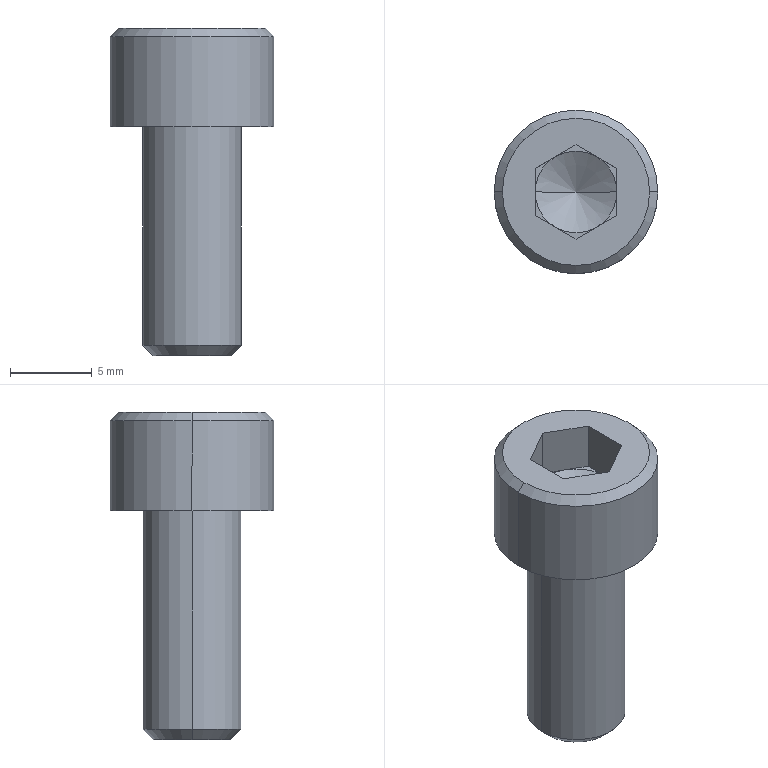Part | NX | features BREP 1 | 1 solid | 25 faces | box 10 x 10 x 20 mm | volume 785.579 mm3 | plane 15 | cone 6 | cylinder 4 | commonest cylinder face diameters 6 x2 10 x2
STEP:
#1=CARTESIAN_POINT('',(0.,0.,1.557));
#2=VERTEX_POINT('',#1);
#3=CARTESIAN_POINT('',(2.5,0.,3.));
#4=VERTEX_POINT('',#3);
#5=CARTESIAN_POINT('',(0.,0.,1.557));
#6=DIRECTION('',(0.866,0.,0.5));
#7=VECTOR('',#6,1000.);
#8=LINE('',#5,#7);
#9=EDGE_CURVE('',#2,#4,#8,.T.);
#10=ORIENTED_EDGE('',*,*,#9,.F.);
#11=CARTESIAN_POINT('',(-2.5,0.,3.));
#12=VERTEX_POINT('',#11);
#13=CARTESIAN_POINT('',(0.,0.,1.557));
#14=DIRECTION('',(-0.866,0.,0.5));
#15=VECTOR('',#14,1000.);
#16=LINE('',#13,#15);
#17=EDGE_CURVE('',#2,#12,#16,.T.);
#18=ORIENTED_EDGE('',*,*,#17,.T.);
#19=CARTESIAN_POINT('',(-1.25,-2.165,3.));
#20=VERTEX_POINT('',#19);
#21=CARTESIAN_POINT('',(0.,0.,3.));
#22=DIRECTION('',(0.,0.,1.));
#23=DIRECTION('',(1.,0.,0.));
#24=AXIS2_PLACEMENT_3D('',#21,#22,#23);
#25=CIRCLE('',#24,2.5);
#26=EDGE_CURVE('',#12,#20,#25,.T.);
#27=ORIENTED_EDGE('',*,*,#26,.T.);
#28=CARTESIAN_POINT('',(1.25,-2.165,3.));
#29=VERTEX_POINT('',#28);
#30=CARTESIAN_POINT('',(0.,0.,3.));
#31=DIRECTION('',(0.,0.,1.));
#32=DIRECTION('',(1.,0.,0.));
#33=AXIS2_PLACEMENT_3D('',#30,#31,#32);
#34=CIRCLE('',#33,2.5);
#35=EDGE_CURVE('',#20,#29,#34,.T.);
#36=ORIENTED_EDGE('',*,*,#35,.T.);
#37=CARTESIAN_POINT('',(0.,0.,3.));
#38=DIRECTION('',(0.,0.,1.));
#39=DIRECTION('',(1.,0.,0.));
#40=AXIS2_PLACEMENT_3D('',#37,#38,#39);
#41=CIRCLE('',#40,2.5);
#42=EDGE_CURVE('',#29,#4,#41,.T.);
#43=ORIENTED_EDGE('',*,*,#42,.T.);
#44=EDGE_LOOP('',(#10,#18,#27,#36,#43));
#45=FACE_BOUND('',#44,.T.);
#46=CARTESIAN_POINT('',(0.,0.,1001.557));
#47=DIRECTION('',(0.,0.,1.));
#48=DIRECTION('',(-1.,0.,0.));
#49=AXIS2_PLACEMENT_3D('',#46,#47,#48);
#50=CONICAL_SURFACE('',#49,1732.051,1.047);
#51=ADVANCED_FACE('',(#45),#50,.F.);
#52=CARTESIAN_POINT('',(5.,0.,0.));
#53=VERTEX_POINT('',#52);
#54=CARTESIAN_POINT('',(-5.,0.,0.));
#55=VERTEX_POINT('',#54);
#56=CARTESIAN_POINT('',(0.,0.,0.));
#57=DIRECTION('',(0.,0.,1.));
#58=DIRECTION('',(1.,0.,0.));
#59=AXIS2_PLACEMENT_3D('',#56,#57,#58);
#60=CIRCLE('',#59,5.);
#61=EDGE_CURVE('',#53,#55,#60,.T.);
#62=ORIENTED_EDGE('',*,*,#61,.T.);
#63=CARTESIAN_POINT('',(-5.,0.,5.5));
#64=VERTEX_POINT('',#63);
#65=CARTESIAN_POINT('',(-5.,0.,0.));
#66=DIRECTION('',(0.,0.,1.));
#67=VECTOR('',#66,1000.);
#68=LINE('',#65,#67);
#69=EDGE_CURVE('',#55,#64,#68,.T.);
#70=ORIENTED_EDGE('',*,*,#69,.T.);
#71=CARTESIAN_POINT('',(5.,0.,5.5));
#72=VERTEX_POINT('',#71);
#73=CARTESIAN_POINT('',(0.,0.,5.5));
#74=DIRECTION('',(0.,0.,1.));
#75=DIRECTION('',(1.,0.,0.));
#76=AXIS2_PLACEMENT_3D('',#73,#74,#75);
#77=CIRCLE('',#76,5.);
#78=EDGE_CURVE('',#72,#64,#77,.T.);
#79=ORIENTED_EDGE('',*,*,#78,.F.);
#80=CARTESIAN_POINT('',(5.,0.,0.));
#81=DIRECTION('',(0.,0.,1.));
#82=VECTOR('',#81,1000.);
#83=LINE('',#80,#82);
#84=EDGE_CURVE('',#53,#72,#83,.T.);
#85=ORIENTED_EDGE('',*,*,#84,.F.);
#86=EDGE_LOOP('',(#62,#70,#79,#85));
#87=FACE_BOUND('',#86,.T.);
#88=CARTESIAN_POINT('',(0.,0.,0.));
#89=DIRECTION('',(0.,0.,1.));
#90=DIRECTION('',(-1.,0.,0.));
#91=AXIS2_PLACEMENT_3D('',#88,#89,#90);
#92=CYLINDRICAL_SURFACE('',#91,5.);
#93=ADVANCED_FACE('',(#87),#92,.T.);
#94=CARTESIAN_POINT('',(4.5,0.,6.));
#95=VERTEX_POINT('',#94);
#96=CARTESIAN_POINT('',(-4.5,0.,6.));
#97=VERTEX_POINT('',#96);
#98=CARTESIAN_POINT('',(0.,0.,6.));
#99=DIRECTION('',(0.,0.,1.));
#100=DIRECTION('',(1.,0.,0.));
#101=AXIS2_PLACEMENT_3D('',#98,#99,#100);
#102=CIRCLE('',#101,4.5);
#103=EDGE_CURVE('',#95,#97,#102,.T.);
#104=ORIENTED_EDGE('',*,*,#103,.F.);
#105=CARTESIAN_POINT('',(5.,0.,5.5));
#106=DIRECTION('',(0.7071,0.,-0.7071));
#107=VECTOR('',#106,1000.);
#108=LINE('',#105,#107);
#109=EDGE_CURVE('',#72,#95,#108,.F.);
#110=ORIENTED_EDGE('',*,*,#109,.F.);
#111=ORIENTED_EDGE('',*,*,#78,.T.);
#112=CARTESIAN_POINT('',(-5.,0.,5.5));
#113=DIRECTION('',(-0.7071,0.,-0.7071));
#114=VECTOR('',#113,1000.);
#115=LINE('',#112,#114);
#116=EDGE_CURVE('',#64,#97,#115,.F.);
#117=ORIENTED_EDGE('',*,*,#116,.T.);
#118=EDGE_LOOP('',(#104,#110,#111,#117));
#119=FACE_BOUND('',#118,.T.);
#120=CARTESIAN_POINT('',(0.,0.,5.5));
#121=DIRECTION('',(0.,0.,-1.));
#122=DIRECTION('',(1.,0.,0.));
#123=AXIS2_PLACEMENT_3D('',#120,#121,#122);
#124=CONICAL_SURFACE('',#123,5.,0.7854);
#125=ADVANCED_FACE('',(#119),#124,.T.);
#126=CARTESIAN_POINT('',(2.386,0.,-14.));
#127=VERTEX_POINT('',#126);
#128=CARTESIAN_POINT('',(-2.386,0.,-14.));
#129=VERTEX_POINT('',#128);
#130=CARTESIAN_POINT('',(0.,0.,-14.));
#131=DIRECTION('',(0.,0.,1.));
#132=DIRECTION('',(1.,0.,0.));
#133=AXIS2_PLACEMENT_3D('',#130,#131,#132);
#134=CIRCLE('',#133,2.386);
#135=EDGE_CURVE('',#127,#129,#134,.T.);
#136=ORIENTED_EDGE('',*,*,#135,.T.);
#137=CARTESIAN_POINT('',(-3.,0.,-13.386));
#138=VERTEX_POINT('',#137);
#139=CARTESIAN_POINT('',(-2.386,0.,-14.));
#140=DIRECTION('',(-0.7071,0.,0.7071));
#141=VECTOR('',#140,1000.);
#142=LINE('',#139,#141);
#143=EDGE_CURVE('',#129,#138,#142,.T.);
#144=ORIENTED_EDGE('',*,*,#143,.T.);
#145=CARTESIAN_POINT('',(3.,0.,-13.386));
#146=VERTEX_POINT('',#145);
#147=CARTESIAN_POINT('',(0.,0.,-13.386));
#148=DIRECTION('',(0.,0.,1.));
#149=DIRECTION('',(1.,0.,0.));
#150=AXIS2_PLACEMENT_3D('',#147,#148,#149);
#151=CIRCLE('',#150,3.);
#152=EDGE_CURVE('',#146,#138,#151,.T.);
#153=ORIENTED_EDGE('',*,*,#152,.F.);
#154=CARTESIAN_POINT('',(2.386,0.,-14.));
#155=DIRECTION('',(0.7071,0.,0.7071));
#156=VECTOR('',#155,1000.);
#157=LINE('',#154,#156);
#158=EDGE_CURVE('',#127,#146,#157,.T.);
#159=ORIENTED_EDGE('',*,*,#158,.F.);
#160=EDGE_LOOP('',(#136,#144,#153,#159));
#161=FACE_BOUND('',#160,.T.);
#162=CARTESIAN_POINT('',(0.,0.,-14.));
#163=DIRECTION('',(0.,0.,1.));
#164=DIRECTION('',(-1.,0.,0.));
#165=AXIS2_PLACEMENT_3D('',#162,#163,#164);
#166=CONICAL_SURFACE('',#165,2.386,0.7854);
#167=ADVANCED_FACE('',(#161),#166,.T.);
#168=ORIENTED_EDGE('',*,*,#152,.T.);
#169=CARTESIAN_POINT('',(-3.,0.,0.));
#170=VERTEX_POINT('',#169);
#171=CARTESIAN_POINT('',(-3.,0.,-14.));
#172=DIRECTION('',(0.,0.,1.));
#173=VECTOR('',#172,1000.);
#174=LINE('',#171,#173);
#175=EDGE_CURVE('',#138,#170,#174,.T.);
#176=ORIENTED_EDGE('',*,*,#175,.T.);
#177=CARTESIAN_POINT('',(3.,0.,0.));
#178=VERTEX_POINT('',#177);
#179=CARTESIAN_POINT('',(0.,0.,0.));
#180=DIRECTION('',(0.,0.,1.));
#181=DIRECTION('',(1.,0.,0.));
#182=AXIS2_PLACEMENT_3D('',#179,#180,#181);
#183=CIRCLE('',#182,3.);
#184=EDGE_CURVE('',#178,#170,#183,.T.);
#185=ORIENTED_EDGE('',*,*,#184,.F.);
#186=CARTESIAN_POINT('',(3.,0.,-14.));
#187=DIRECTION('',(0.,0.,1.));
#188=VECTOR('',#187,1000.);
#189=LINE('',#186,#188);
#190=EDGE_CURVE('',#146,#178,#189,.T.);
#191=ORIENTED_EDGE('',*,*,#190,.F.);
#192=EDGE_LOOP('',(#168,#176,#185,#191));
#193=FACE_BOUND('',#192,.T.);
#194=CARTESIAN_POINT('',(0.,0.,-14.));
#195=DIRECTION('',(0.,0.,1.));
#196=DIRECTION('',(-1.,0.,0.));
#197=AXIS2_PLACEMENT_3D('',#194,#195,#196);
#198=CYLINDRICAL_SURFACE('',#197,3.);
#199=ADVANCED_FACE('',(#193),#198,.T.);
#200=CARTESIAN_POINT('',(1.25,2.165,3.));
#201=VERTEX_POINT('',#200);
#202=CARTESIAN_POINT('',(0.,0.,3.));
#203=DIRECTION('',(0.,0.,1.));
#204=DIRECTION('',(1.,0.,0.));
#205=AXIS2_PLACEMENT_3D('',#202,#203,#204);
#206=CIRCLE('',#205,2.5);
#207=EDGE_CURVE('',#4,#201,#206,.T.);
#208=ORIENTED_EDGE('',*,*,#207,.F.);
#209=CARTESIAN_POINT('',(2.5,1.443,3.));
#210=VERTEX_POINT('',#209);
#211=CARTESIAN_POINT('',(2.5,-1.443,3.));
#212=DIRECTION('',(0.,1.,0.));
#213=VECTOR('',#212,1000.);
#214=LINE('',#211,#213);
#215=EDGE_CURVE('',#4,#210,#214,.T.);
#216=ORIENTED_EDGE('',*,*,#215,.T.);
#217=CARTESIAN_POINT('',(2.5,1.443,3.));
#218=DIRECTION('',(-0.866,0.5,0.));
#219=VECTOR('',#218,1000.);
#220=LINE('',#217,#219);
#221=EDGE_CURVE('',#210,#201,#220,.T.);
#222=ORIENTED_EDGE('',*,*,#221,.T.);
#223=EDGE_LOOP('',(#208,#216,#222));
#224=FACE_BOUND('',#223,.T.);
#225=CARTESIAN_POINT('',(0.,0.,3.));
#226=DIRECTION('',(0.,0.,1.));
#227=DIRECTION('',(-1.,0.,0.));
#228=AXIS2_PLACEMENT_3D('',#225,#226,#227);
#229=PLANE('',#228);
#230=ADVANCED_FACE('',(#224),#229,.T.);
#231=CARTESIAN_POINT('',(-1.25,2.165,3.));
#232=VERTEX_POINT('',#231);
#233=CARTESIAN_POINT('',(0.,0.,3.));
#234=DIRECTION('',(0.,0.,1.));
#235=DIRECTION('',(1.,0.,0.));
#236=AXIS2_PLACEMENT_3D('',#233,#234,#235);
#237=CIRCLE('',#236,2.5);
#238=EDGE_CURVE('',#201,#232,#237,.T.);
#239=ORIENTED_EDGE('',*,*,#238,.F.);
#240=CARTESIAN_POINT('',(0.,2.887,3.));
#241=VERTEX_POINT('',#240);
#242=CARTESIAN_POINT('',(2.5,1.443,3.));
#243=DIRECTION('',(-0.866,0.5,0.));
#244=VECTOR('',#243,1000.);
#245=LINE('',#242,#244);
#246=EDGE_CURVE('',#201,#241,#245,.T.);
#247=ORIENTED_EDGE('',*,*,#246,.T.);
#248=CARTESIAN_POINT('',(0.,2.887,3.));
#249=DIRECTION('',(-0.866,-0.5,0.));
#250=VECTOR('',#249,1000.);
#251=LINE('',#248,#250);
#252=EDGE_CURVE('',#241,#232,#251,.T.);
#253=ORIENTED_EDGE('',*,*,#252,.T.);
#254=EDGE_LOOP('',(#239,#247,#253));
#255=FACE_BOUND('',#254,.T.);
#256=CARTESIAN_POINT('',(0.,0.,3.));
#257=DIRECTION('',(0.,0.,1.));
#258=DIRECTION('',(-1.,0.,0.));
#259=AXIS2_PLACEMENT_3D('',#256,#257,#258);
#260=PLANE('',#259);
#261=ADVANCED_FACE('',(#255),#260,.T.);
#262=CARTESIAN_POINT('',(0.,0.,3.));
#263=DIRECTION('',(0.,0.,1.));
#264=DIRECTION('',(1.,0.,0.));
#265=AXIS2_PLACEMENT_3D('',#262,#263,#264);
#266=CIRCLE('',#265,2.5);
#267=EDGE_CURVE('',#232,#12,#266,.T.);
#268=ORIENTED_EDGE('',*,*,#267,.F.);
#269=CARTESIAN_POINT('',(-2.5,1.443,3.));
#270=VERTEX_POINT('',#269);
#271=CARTESIAN_POINT('',(0.,2.887,3.));
#272=DIRECTION('',(-0.866,-0.5,0.));
#273=VECTOR('',#272,1000.);
#274=LINE('',#271,#273);
#275=EDGE_CURVE('',#232,#270,#274,.T.);
#276=ORIENTED_EDGE('',*,*,#275,.T.);
#277=CARTESIAN_POINT('',(-2.5,1.443,3.));
#278=DIRECTION('',(0.,-1.,0.));
#279=VECTOR('',#278,1000.);
#280=LINE('',#277,#279);
#281=EDGE_CURVE('',#270,#12,#280,.T.);
#282=ORIENTED_EDGE('',*,*,#281,.T.);
#283=EDGE_LOOP('',(#268,#276,#282));
#284=FACE_BOUND('',#283,.T.);
#285=CARTESIAN_POINT('',(0.,0.,3.));
#286=DIRECTION('',(0.,0.,1.));
#287=DIRECTION('',(-1.,0.,0.));
#288=AXIS2_PLACEMENT_3D('',#285,#286,#287);
#289=PLANE('',#288);
#290=ADVANCED_FACE('',(#284),#289,.T.);
#291=ORIENTED_EDGE('',*,*,#26,.F.);
#292=CARTESIAN_POINT('',(-2.5,-1.443,3.));
#293=VERTEX_POINT('',#292);
#294=CARTESIAN_POINT('',(-2.5,1.443,3.));
#295=DIRECTION('',(0.,-1.,0.));
#296=VECTOR('',#295,1000.);
#297=LINE('',#294,#296);
#298=EDGE_CURVE('',#12,#293,#297,.T.);
#299=ORIENTED_EDGE('',*,*,#298,.T.);
#300=CARTESIAN_POINT('',(-2.5,-1.443,3.));
#301=DIRECTION('',(0.866,-0.5,0.));
#302=VECTOR('',#301,1000.);
#303=LINE('',#300,#302);
#304=EDGE_CURVE('',#293,#20,#303,.T.);
#305=ORIENTED_EDGE('',*,*,#304,.T.);
#306=EDGE_LOOP('',(#291,#299,#305));
#307=FACE_BOUND('',#306,.T.);
#308=CARTESIAN_POINT('',(0.,0.,3.));
#309=DIRECTION('',(0.,0.,1.));
#310=DIRECTION('',(-1.,0.,0.));
#311=AXIS2_PLACEMENT_3D('',#308,#309,#310);
#312=PLANE('',#311);
#313=ADVANCED_FACE('',(#307),#312,.T.);
#314=ORIENTED_EDGE('',*,*,#35,.F.);
#315=CARTESIAN_POINT('',(0.,-2.887,3.));
#316=VERTEX_POINT('',#315);
#317=CARTESIAN_POINT('',(-2.5,-1.443,3.));
#318=DIRECTION('',(0.866,-0.5,0.));
#319=VECTOR('',#318,1000.);
#320=LINE('',#317,#319);
#321=EDGE_CURVE('',#20,#316,#320,.T.);
#322=ORIENTED_EDGE('',*,*,#321,.T.);
#323=CARTESIAN_POINT('',(0.,-2.887,3.));
#324=DIRECTION('',(0.866,0.5,0.));
#325=VECTOR('',#324,1000.);
#326=LINE('',#323,#325);
#327=EDGE_CURVE('',#316,#29,#326,.T.);
#328=ORIENTED_EDGE('',*,*,#327,.T.);
#329=EDGE_LOOP('',(#314,#322,#328));
#330=FACE_BOUND('',#329,.T.);
#331=CARTESIAN_POINT('',(0.,0.,3.));
#332=DIRECTION('',(0.,0.,1.));
#333=DIRECTION('',(-1.,0.,0.));
#334=AXIS2_PLACEMENT_3D('',#331,#332,#333);
#335=PLANE('',#334);
#336=ADVANCED_FACE('',(#330),#335,.T.);
#337=ORIENTED_EDGE('',*,*,#175,.F.);
#338=CARTESIAN_POINT('',(0.,0.,-13.386));
#339=DIRECTION('',(0.,0.,1.));
#340=DIRECTION('',(1.,0.,0.));
#341=AXIS2_PLACEMENT_3D('',#338,#339,#340);
#342=CIRCLE('',#341,3.);
#343=EDGE_CURVE('',#138,#146,#342,.T.);
#344=ORIENTED_EDGE('',*,*,#343,.T.);
#345=ORIENTED_EDGE('',*,*,#190,.T.);
#346=CARTESIAN_POINT('',(0.,0.,0.));
#347=DIRECTION('',(0.,0.,1.));
#348=DIRECTION('',(1.,0.,0.));
#349=AXIS2_PLACEMENT_3D('',#346,#347,#348);
#350=CIRCLE('',#349,3.);
#351=EDGE_CURVE('',#170,#178,#350,.T.);
#352=ORIENTED_EDGE('',*,*,#351,.F.);
#353=EDGE_LOOP('',(#337,#344,#345,#352));
#354=FACE_BOUND('',#353,.T.);
#355=CARTESIAN_POINT('',(0.,0.,-14.));
#356=DIRECTION('',(0.,0.,1.));
#357=DIRECTION('',(-1.,0.,0.));
#358=AXIS2_PLACEMENT_3D('',#355,#356,#357);
#359=CYLINDRICAL_SURFACE('',#358,3.);
#360=ADVANCED_FACE('',(#354),#359,.T.);
#361=ORIENTED_EDGE('',*,*,#143,.F.);
#362=CARTESIAN_POINT('',(0.,0.,-14.));
#363=DIRECTION('',(0.,0.,1.));
#364=DIRECTION('',(1.,0.,0.));
#365=AXIS2_PLACEMENT_3D('',#362,#363,#364);
#366=CIRCLE('',#365,2.386);
#367=EDGE_CURVE('',#129,#127,#366,.T.);
#368=ORIENTED_EDGE('',*,*,#367,.T.);
#369=ORIENTED_EDGE('',*,*,#158,.T.);
#370=ORIENTED_EDGE('',*,*,#343,.F.);
#371=EDGE_LOOP('',(#361,#368,#369,#370));
#372=FACE_BOUND('',#371,.T.);
#373=CARTESIAN_POINT('',(0.,0.,-14.));
#374=DIRECTION('',(0.,0.,1.));
#375=DIRECTION('',(-1.,0.,0.));
#376=AXIS2_PLACEMENT_3D('',#373,#374,#375);
#377=CONICAL_SURFACE('',#376,2.386,0.7854);
#378=ADVANCED_FACE('',(#372),#377,.T.);
#379=ORIENTED_EDGE('',*,*,#135,.F.);
#380=ORIENTED_EDGE('',*,*,#367,.F.);
#381=EDGE_LOOP('',(#379,#380));
#382=FACE_BOUND('',#381,.T.);
#383=CARTESIAN_POINT('',(0.,2.386,-14.));
#384=DIRECTION('',(0.,0.,1.));
#385=DIRECTION('',(-1.,0.,0.));
#386=AXIS2_PLACEMENT_3D('',#383,#384,#385);
#387=PLANE('',#386);
#388=ADVANCED_FACE('',(#382),#387,.F.);
#389=CARTESIAN_POINT('',(0.,-2.887,6.));
#390=VERTEX_POINT('',#389);
#391=CARTESIAN_POINT('',(2.5,-1.443,6.));
#392=VERTEX_POINT('',#391);
#393=CARTESIAN_POINT('',(0.,-2.887,6.));
#394=DIRECTION('',(0.866,0.5,0.));
#395=VECTOR('',#394,1000.);
#396=LINE('',#393,#395);
#397=EDGE_CURVE('',#390,#392,#396,.T.);
#398=ORIENTED_EDGE('',*,*,#397,.F.);
#399=CARTESIAN_POINT('',(-2.5,-1.443,6.));
#400=VERTEX_POINT('',#399);
#401=CARTESIAN_POINT('',(-2.5,-1.443,6.));
#402=DIRECTION('',(0.866,-0.5,0.));
#403=VECTOR('',#402,1000.);
#404=LINE('',#401,#403);
#405=EDGE_CURVE('',#400,#390,#404,.T.);
#406=ORIENTED_EDGE('',*,*,#405,.F.);
#407=CARTESIAN_POINT('',(-2.5,1.443,6.));
#408=VERTEX_POINT('',#407);
#409=CARTESIAN_POINT('',(-2.5,1.443,6.));
#410=DIRECTION('',(0.,-1.,0.));
#411=VECTOR('',#410,1000.);
#412=LINE('',#409,#411);
#413=EDGE_CURVE('',#408,#400,#412,.T.);
#414=ORIENTED_EDGE('',*,*,#413,.F.);
#415=CARTESIAN_POINT('',(0.,2.887,6.));
#416=VERTEX_POINT('',#415);
#417=CARTESIAN_POINT('',(0.,2.887,6.));
#418=DIRECTION('',(-0.866,-0.5,0.));
#419=VECTOR('',#418,1000.);
#420=LINE('',#417,#419);
#421=EDGE_CURVE('',#416,#408,#420,.T.);
#422=ORIENTED_EDGE('',*,*,#421,.F.);
#423=CARTESIAN_POINT('',(2.5,1.443,6.));
#424=VERTEX_POINT('',#423);
#425=CARTESIAN_POINT('',(2.5,1.443,6.));
#426=DIRECTION('',(-0.866,0.5,0.));
#427=VECTOR('',#426,1000.);
#428=LINE('',#425,#427);
#429=EDGE_CURVE('',#424,#416,#428,.T.);
#430=ORIENTED_EDGE('',*,*,#429,.F.);
#431=CARTESIAN_POINT('',(2.5,-1.443,6.));
#432=DIRECTION('',(0.,1.,0.));
#433=VECTOR('',#432,1000.);
#434=LINE('',#431,#433);
#435=EDGE_CURVE('',#392,#424,#434,.T.);
#436=ORIENTED_EDGE('',*,*,#435,.F.);
#437=EDGE_LOOP('',(#398,#406,#414,#422,#430,#436));
#438=FACE_BOUND('',#437,.T.);
#439=CARTESIAN_POINT('',(0.,0.,6.));
#440=DIRECTION('',(0.,0.,1.));
#441=DIRECTION('',(1.,0.,0.));
#442=AXIS2_PLACEMENT_3D('',#439,#440,#441);
#443=CIRCLE('',#442,4.5);
#444=EDGE_CURVE('',#97,#95,#443,.T.);
#445=ORIENTED_EDGE('',*,*,#444,.T.);
#446=ORIENTED_EDGE('',*,*,#103,.T.);
#447=EDGE_LOOP('',(#445,#446));
#448=FACE_BOUND('',#447,.T.);
#449=CARTESIAN_POINT('',(0.,0.,6.));
#450=DIRECTION('',(0.,0.,-1.));
#451=DIRECTION('',(1.,0.,0.));
#452=AXIS2_PLACEMENT_3D('',#449,#450,#451);
#453=PLANE('',#452);
#454=ADVANCED_FACE('',(#438,#448),#453,.F.);
#455=ORIENTED_EDGE('',*,*,#109,.T.);
#456=ORIENTED_EDGE('',*,*,#444,.F.);
#457=ORIENTED_EDGE('',*,*,#116,.F.);
#458=CARTESIAN_POINT('',(0.,0.,5.5));
#459=DIRECTION('',(0.,0.,1.));
#460=DIRECTION('',(1.,0.,0.));
#461=AXIS2_PLACEMENT_3D('',#458,#459,#460);
#462=CIRCLE('',#461,5.);
#463=EDGE_CURVE('',#64,#72,#462,.T.);
#464=ORIENTED_EDGE('',*,*,#463,.T.);
#465=EDGE_LOOP('',(#455,#456,#457,#464));
#466=FACE_BOUND('',#465,.T.);
#467=CARTESIAN_POINT('',(0.,0.,5.5));
#468=DIRECTION('',(0.,0.,-1.));
#469=DIRECTION('',(1.,0.,0.));
#470=AXIS2_PLACEMENT_3D('',#467,#468,#469);
#471=CONICAL_SURFACE('',#470,5.,0.7854);
#472=ADVANCED_FACE('',(#466),#471,.T.);
#473=ORIENTED_EDGE('',*,*,#69,.F.);
#474=CARTESIAN_POINT('',(0.,0.,0.));
#475=DIRECTION('',(0.,0.,1.));
#476=DIRECTION('',(1.,0.,0.));
#477=AXIS2_PLACEMENT_3D('',#474,#475,#476);
#478=CIRCLE('',#477,5.);
#479=EDGE_CURVE('',#55,#53,#478,.T.);
#480=ORIENTED_EDGE('',*,*,#479,.T.);
#481=ORIENTED_EDGE('',*,*,#84,.T.);
#482=ORIENTED_EDGE('',*,*,#463,.F.);
#483=EDGE_LOOP('',(#473,#480,#481,#482));
#484=FACE_BOUND('',#483,.T.);
#485=CARTESIAN_POINT('',(0.,0.,0.));
#486=DIRECTION('',(0.,0.,1.));
#487=DIRECTION('',(-1.,0.,0.));
#488=AXIS2_PLACEMENT_3D('',#485,#486,#487);
#489=CYLINDRICAL_SURFACE('',#488,5.);
#490=ADVANCED_FACE('',(#484),#489,.T.);
#491=ORIENTED_EDGE('',*,*,#184,.T.);
#492=ORIENTED_EDGE('',*,*,#351,.T.);
#493=EDGE_LOOP('',(#491,#492));
#494=FACE_BOUND('',#493,.T.);
#495=ORIENTED_EDGE('',*,*,#61,.F.);
#496=ORIENTED_EDGE('',*,*,#479,.F.);
#497=EDGE_LOOP('',(#495,#496));
#498=FACE_BOUND('',#497,.T.);
#499=CARTESIAN_POINT('',(0.,5.,0.));
#500=DIRECTION('',(0.,0.,1.));
#501=DIRECTION('',(-1.,0.,0.));
#502=AXIS2_PLACEMENT_3D('',#499,#500,#501);
#503=PLANE('',#502);
#504=ADVANCED_FACE('',(#494,#498),#503,.F.);
#505=ORIENTED_EDGE('',*,*,#405,.T.);
#506=CARTESIAN_POINT('',(0.,-2.887,3.));
#507=DIRECTION('',(0.,0.,1.));
#508=VECTOR('',#507,1000.);
#509=LINE('',#506,#508);
#510=EDGE_CURVE('',#316,#390,#509,.T.);
#511=ORIENTED_EDGE('',*,*,#510,.F.);
#512=ORIENTED_EDGE('',*,*,#321,.F.);
#513=ORIENTED_EDGE('',*,*,#304,.F.);
#514=CARTESIAN_POINT('',(-2.5,-1.443,3.));
#515=DIRECTION('',(0.,0.,1.));
#516=VECTOR('',#515,1000.);
#517=LINE('',#514,#516);
#518=EDGE_CURVE('',#293,#400,#517,.T.);
#519=ORIENTED_EDGE('',*,*,#518,.T.);
#520=EDGE_LOOP('',(#505,#511,#512,#513,#519));
#521=FACE_BOUND('',#520,.T.);
#522=CARTESIAN_POINT('',(-2.5,-1.443,3.));
#523=DIRECTION('',(-0.5,-0.866,0.));
#524=DIRECTION('',(-0.866,0.5,0.));
#525=AXIS2_PLACEMENT_3D('',#522,#523,#524);
#526=PLANE('',#525);
#527=ADVANCED_FACE('',(#521),#526,.F.);
#528=ORIENTED_EDGE('',*,*,#413,.T.);
#529=ORIENTED_EDGE('',*,*,#518,.F.);
#530=ORIENTED_EDGE('',*,*,#298,.F.);
#531=ORIENTED_EDGE('',*,*,#281,.F.);
#532=CARTESIAN_POINT('',(-2.5,1.443,3.));
#533=DIRECTION('',(0.,0.,1.));
#534=VECTOR('',#533,1000.);
#535=LINE('',#532,#534);
#536=EDGE_CURVE('',#270,#408,#535,.T.);
#537=ORIENTED_EDGE('',*,*,#536,.T.);
#538=EDGE_LOOP('',(#528,#529,#530,#531,#537));
#539=FACE_BOUND('',#538,.T.);
#540=CARTESIAN_POINT('',(-2.5,1.443,3.));
#541=DIRECTION('',(-1.,0.,0.));
#542=DIRECTION('',(0.,0.,-1.));
#543=AXIS2_PLACEMENT_3D('',#540,#541,#542);
#544=PLANE('',#543);
#545=ADVANCED_FACE('',(#539),#544,.F.);
#546=ORIENTED_EDGE('',*,*,#421,.T.);
#547=ORIENTED_EDGE('',*,*,#536,.F.);
#548=ORIENTED_EDGE('',*,*,#275,.F.);
#549=ORIENTED_EDGE('',*,*,#252,.F.);
#550=CARTESIAN_POINT('',(0.,2.887,3.));
#551=DIRECTION('',(0.,0.,1.));
#552=VECTOR('',#551,1000.);
#553=LINE('',#550,#552);
#554=EDGE_CURVE('',#241,#416,#553,.T.);
#555=ORIENTED_EDGE('',*,*,#554,.T.);
#556=EDGE_LOOP('',(#546,#547,#548,#549,#555));
#557=FACE_BOUND('',#556,.T.);
#558=CARTESIAN_POINT('',(0.,2.887,3.));
#559=DIRECTION('',(-0.5,0.866,0.));
#560=DIRECTION('',(0.866,0.5,0.));
#561=AXIS2_PLACEMENT_3D('',#558,#559,#560);
#562=PLANE('',#561);
#563=ADVANCED_FACE('',(#557),#562,.F.);
#564=ORIENTED_EDGE('',*,*,#429,.T.);
#565=ORIENTED_EDGE('',*,*,#554,.F.);
#566=ORIENTED_EDGE('',*,*,#246,.F.);
#567=ORIENTED_EDGE('',*,*,#221,.F.);
#568=CARTESIAN_POINT('',(2.5,1.443,3.));
#569=DIRECTION('',(0.,0.,1.));
#570=VECTOR('',#569,1000.);
#571=LINE('',#568,#570);
#572=EDGE_CURVE('',#210,#424,#571,.T.);
#573=ORIENTED_EDGE('',*,*,#572,.T.);
#574=EDGE_LOOP('',(#564,#565,#566,#567,#573));
#575=FACE_BOUND('',#574,.T.);
#576=CARTESIAN_POINT('',(2.5,1.443,3.));
#577=DIRECTION('',(0.5,0.866,0.));
#578=DIRECTION('',(0.866,-0.5,0.));
#579=AXIS2_PLACEMENT_3D('',#576,#577,#578);
#580=PLANE('',#579);
#581=ADVANCED_FACE('',(#575),#580,.F.);
#582=ORIENTED_EDGE('',*,*,#435,.T.);
#583=ORIENTED_EDGE('',*,*,#572,.F.);
#584=ORIENTED_EDGE('',*,*,#215,.F.);
#585=CARTESIAN_POINT('',(2.5,-1.443,3.));
#586=VERTEX_POINT('',#585);
#587=CARTESIAN_POINT('',(2.5,-1.443,3.));
#588=DIRECTION('',(0.,1.,0.));
#589=VECTOR('',#588,1000.);
#590=LINE('',#587,#589);
#591=EDGE_CURVE('',#586,#4,#590,.T.);
#592=ORIENTED_EDGE('',*,*,#591,.F.);
#593=CARTESIAN_POINT('',(2.5,-1.443,3.));
#594=DIRECTION('',(0.,0.,1.));
#595=VECTOR('',#594,1000.);
#596=LINE('',#593,#595);
#597=EDGE_CURVE('',#586,#392,#596,.T.);
#598=ORIENTED_EDGE('',*,*,#597,.T.);
#599=EDGE_LOOP('',(#582,#583,#584,#592,#598));
#600=FACE_BOUND('',#599,.T.);
#601=CARTESIAN_POINT('',(2.5,-1.443,3.));
#602=DIRECTION('',(1.,0.,0.));
#603=DIRECTION('',(0.,0.,1.));
#604=AXIS2_PLACEMENT_3D('',#601,#602,#603);
#605=PLANE('',#604);
#606=ADVANCED_FACE('',(#600),#605,.F.);
#607=ORIENTED_EDGE('',*,*,#397,.T.);
#608=ORIENTED_EDGE('',*,*,#597,.F.);
#609=CARTESIAN_POINT('',(0.,-2.887,3.));
#610=DIRECTION('',(0.866,0.5,0.));
#611=VECTOR('',#610,1000.);
#612=LINE('',#609,#611);
#613=EDGE_CURVE('',#29,#586,#612,.T.);
#614=ORIENTED_EDGE('',*,*,#613,.F.);
#615=ORIENTED_EDGE('',*,*,#327,.F.);
#616=ORIENTED_EDGE('',*,*,#510,.T.);
#617=EDGE_LOOP('',(#607,#608,#614,#615,#616));
#618=FACE_BOUND('',#617,.T.);
#619=CARTESIAN_POINT('',(0.,-2.887,3.));
#620=DIRECTION('',(0.5,-0.866,0.));
#621=DIRECTION('',(-0.866,-0.5,0.));
#622=AXIS2_PLACEMENT_3D('',#619,#620,#621);
#623=PLANE('',#622);
#624=ADVANCED_FACE('',(#618),#623,.F.);
#625=ORIENTED_EDGE('',*,*,#42,.F.);
#626=ORIENTED_EDGE('',*,*,#613,.T.);
#627=ORIENTED_EDGE('',*,*,#591,.T.);
#628=EDGE_LOOP('',(#625,#626,#627));
#629=FACE_BOUND('',#628,.T.);
#630=CARTESIAN_POINT('',(0.,0.,3.));
#631=DIRECTION('',(0.,0.,1.));
#632=DIRECTION('',(-1.,0.,0.));
#633=AXIS2_PLACEMENT_3D('',#630,#631,#632);
#634=PLANE('',#633);
#635=ADVANCED_FACE('',(#629),#634,.T.);
#636=ORIENTED_EDGE('',*,*,#17,.F.);
#637=ORIENTED_EDGE('',*,*,#9,.T.);
#638=ORIENTED_EDGE('',*,*,#207,.T.);
#639=ORIENTED_EDGE('',*,*,#238,.T.);
#640=ORIENTED_EDGE('',*,*,#267,.T.);
#641=EDGE_LOOP('',(#636,#637,#638,#639,#640));
#642=FACE_BOUND('',#641,.T.);
#643=CARTESIAN_POINT('',(0.,0.,1001.557));
#644=DIRECTION('',(0.,0.,1.));
#645=DIRECTION('',(-1.,0.,0.));
#646=AXIS2_PLACEMENT_3D('',#643,#644,#645);
#647=CONICAL_SURFACE('',#646,1732.051,1.047);
#648=ADVANCED_FACE('',(#642),#647,.F.);
#649=CLOSED_SHELL('',(#51,#93,#125,#167,#199,#230,#261,#290,#313,#336,#360,#378,#388,#454,#472,#490,#504,#527,#545,#563,#581,#606,#624,#635,#648));
#650=MANIFOLD_SOLID_BREP('',#649);
#651=(LENGTH_UNIT()NAMED_UNIT(*)SI_UNIT(.MILLI.,.METRE.));
#652=UNCERTAINTY_MEASURE_WITH_UNIT(LENGTH_MEASURE(0.00001),#651,'','');
#653=(NAMED_UNIT(*)PLANE_ANGLE_UNIT()SI_UNIT($,.RADIAN.));
#654=(NAMED_UNIT(*)SI_UNIT($,.STERADIAN.)SOLID_ANGLE_UNIT());
#655=(GEOMETRIC_REPRESENTATION_CONTEXT(3)GLOBAL_UNCERTAINTY_ASSIGNED_CONTEXT((#652))GLOBAL_UNIT_ASSIGNED_CONTEXT((#651,#653,#654))REPRESENTATION_CONTEXT('',''));
#656=ADVANCED_BREP_SHAPE_REPRESENTATION('',(#650),#655);